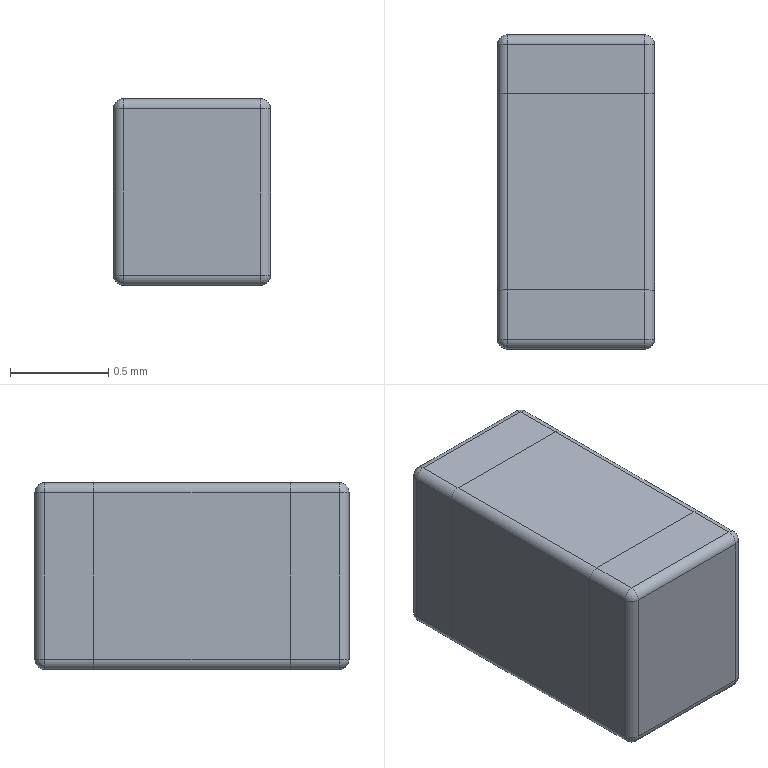Part | STEP file | RJ-USIO-V1_2-220411_1 | 1 solid | 42 faces | box 0.8 x 1.6 x 0.95 mm | volume 1.209 mm3 | cylinder 20 | plane 14 | sphere 8 | commonest cylinder face diameters 0.1 x20